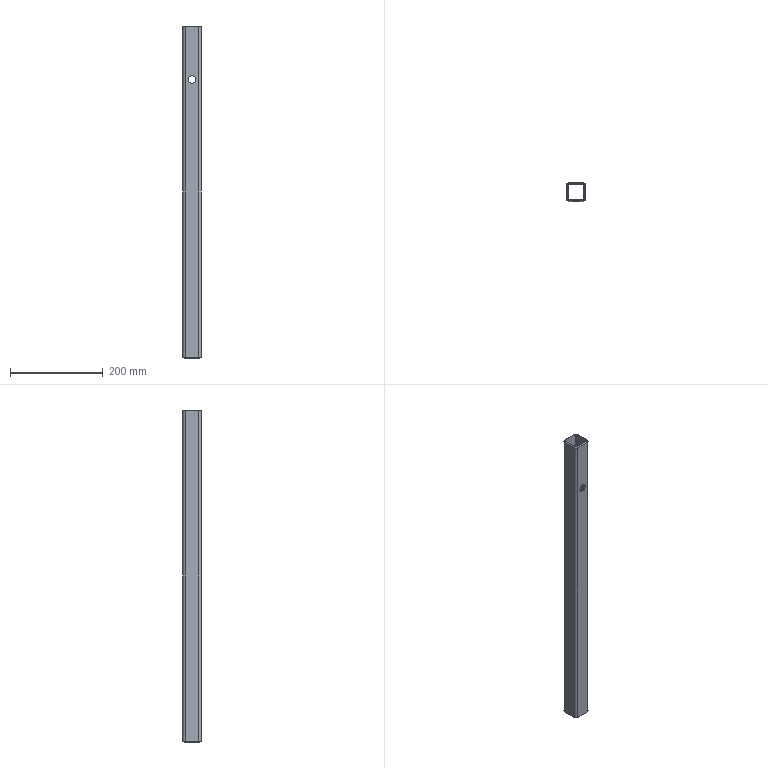Part | STEP file | IN-01-01-01-04 | 1 solid | 38 faces | box 40 x 40 x 715 mm | volume 290473 mm3 | plane 18 | cylinder 12 | cone 8 | commonest cylinder face diameters 5.8 x4 11.6 x4 16 x4